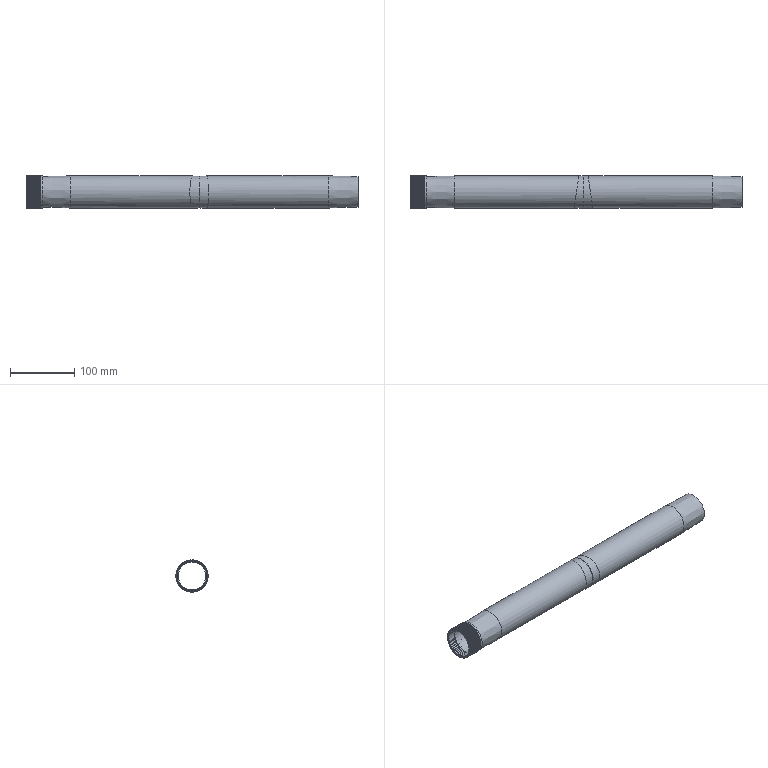Part | STEP file | 6150701 | 1 solid | 2818 faces | box 515 x 50 x 50 mm | volume 250147 mm3 | plane 1607 | cylinder 1209 | cone 2 | commonest cylinder face diameters 0.82 x1200 50 x6 44 x2 43 x1